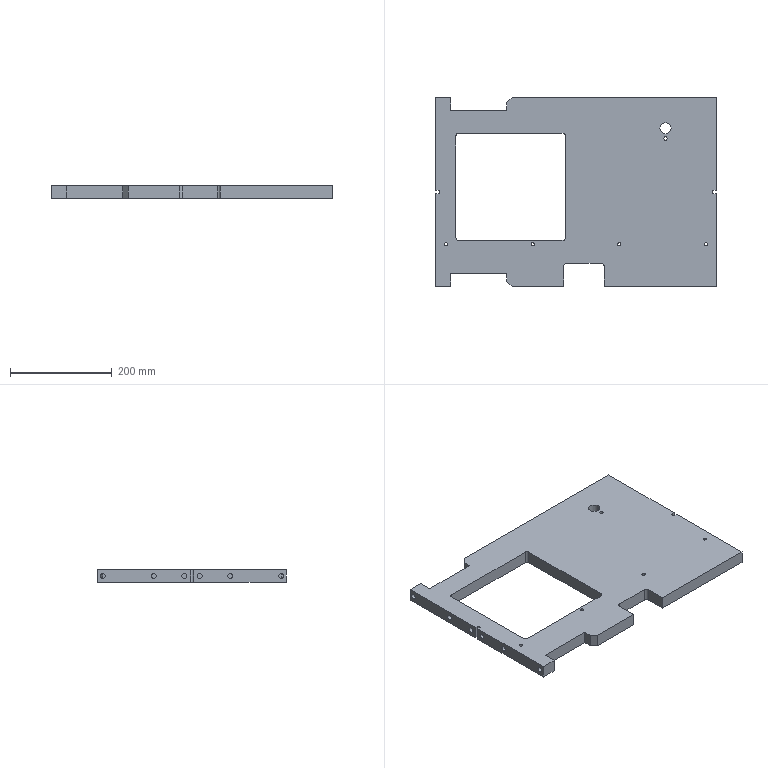Part | 1 solid | 108 faces | box 551 x 370 x 25 mm | volume 3700062 mm3 | cylinder 57 | plane 30 | cone 21 | commonest cylinder face diameters 10 x16 5 x13 6.8 x12 6.5 x10 6 x2 12 x2